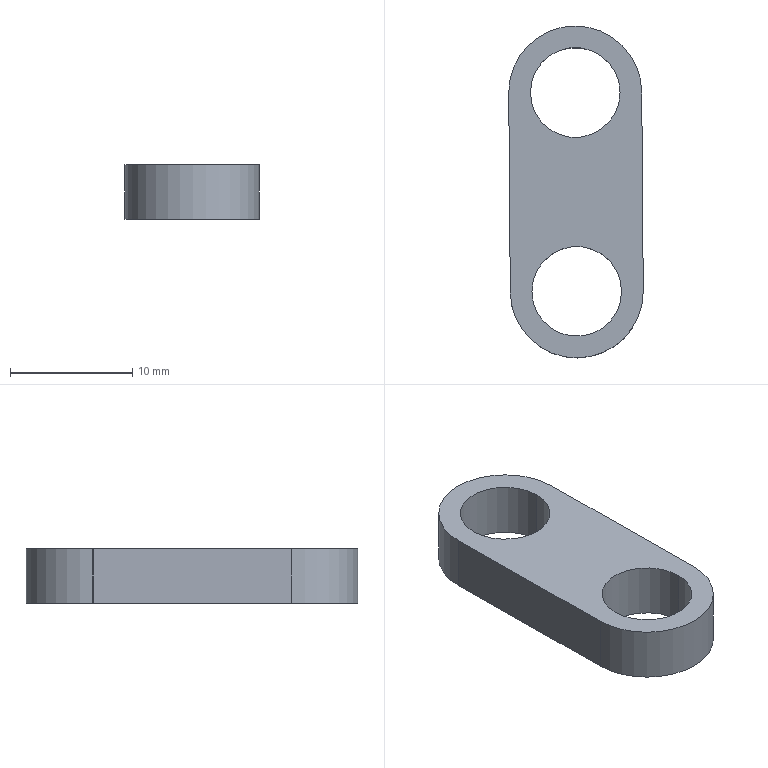Part | SolidWorks | features Extrusion 1 | 1 solid | 11 faces | box 11.013 x 27.178 x 4.5 mm | volume 835.586 mm3 | cylinder 7 | plane 4 | commonest cylinder face diameters 7.349 x4 10.89 x3
STEP:
#1=CARTESIAN_POINT('',(22.577,-16.261,4.5));
#2=VERTEX_POINT('',#1);
#3=CARTESIAN_POINT('',(29.926,-16.261,4.5));
#4=VERTEX_POINT('',#3);
#5=CARTESIAN_POINT('',(26.251,-16.261,4.5));
#6=DIRECTION('',(0.,0.,1.));
#7=DIRECTION('',(1.,0.,0.));
#8=AXIS2_PLACEMENT_3D('',#5,#6,#7);
#9=CIRCLE('',#8,3.675);
#10=EDGE_CURVE('',#2,#4,#9,.T.);
#11=ORIENTED_EDGE('',*,*,#10,.T.);
#12=CARTESIAN_POINT('',(29.926,-16.261,0.));
#13=VERTEX_POINT('',#12);
#14=CARTESIAN_POINT('',(29.926,-16.261,33.825));
#15=DIRECTION('',(0.,0.,-1.));
#16=VECTOR('',#15,1000.);
#17=LINE('',#14,#16);
#18=EDGE_CURVE('',#4,#13,#17,.T.);
#19=ORIENTED_EDGE('',*,*,#18,.T.);
#20=CARTESIAN_POINT('',(22.577,-16.261,0.));
#21=VERTEX_POINT('',#20);
#22=CARTESIAN_POINT('',(26.251,-16.261,0.));
#23=DIRECTION('',(0.,0.,1.));
#24=DIRECTION('',(1.,0.,0.));
#25=AXIS2_PLACEMENT_3D('',#22,#23,#24);
#26=CIRCLE('',#25,3.675);
#27=EDGE_CURVE('',#21,#13,#26,.T.);
#28=ORIENTED_EDGE('',*,*,#27,.F.);
#29=CARTESIAN_POINT('',(22.577,-16.261,33.825));
#30=DIRECTION('',(0.,0.,-1.));
#31=VECTOR('',#30,1000.);
#32=LINE('',#29,#31);
#33=EDGE_CURVE('',#2,#21,#32,.T.);
#34=ORIENTED_EDGE('',*,*,#33,.F.);
#35=EDGE_LOOP('',(#11,#19,#28,#34));
#36=FACE_OUTER_BOUND('',#35,.T.);
#37=CARTESIAN_POINT('',(26.251,-16.261,33.825));
#38=DIRECTION('',(0.,0.,-1.));
#39=DIRECTION('',(-1.,0.,0.));
#40=AXIS2_PLACEMENT_3D('',#37,#38,#39);
#41=CYLINDRICAL_SURFACE('',#40,3.675);
#42=ADVANCED_FACE('',(#36),#41,.F.);
#43=CARTESIAN_POINT('',(20.683,0.027,4.5));
#44=VERTEX_POINT('',#43);
#45=CARTESIAN_POINT('',(20.683,-0.01419,4.5));
#46=VERTEX_POINT('',#45);
#47=CARTESIAN_POINT('',(26.128,0.027,4.5));
#48=DIRECTION('',(0.,0.,1.));
#49=DIRECTION('',(1.,0.,0.));
#50=AXIS2_PLACEMENT_3D('',#47,#48,#49);
#51=CIRCLE('',#50,5.445);
#52=EDGE_CURVE('',#44,#46,#51,.T.);
#53=ORIENTED_EDGE('',*,*,#52,.F.);
#54=CARTESIAN_POINT('',(20.683,0.027,0.));
#55=VERTEX_POINT('',#54);
#56=CARTESIAN_POINT('',(20.683,0.027,33.825));
#57=DIRECTION('',(0.,0.,-1.));
#58=VECTOR('',#57,1000.);
#59=LINE('',#56,#58);
#60=EDGE_CURVE('',#44,#55,#59,.T.);
#61=ORIENTED_EDGE('',*,*,#60,.T.);
#62=CARTESIAN_POINT('',(20.683,-0.01419,0.));
#63=VERTEX_POINT('',#62);
#64=CARTESIAN_POINT('',(26.128,0.027,0.));
#65=DIRECTION('',(0.,0.,1.));
#66=DIRECTION('',(1.,0.,0.));
#67=AXIS2_PLACEMENT_3D('',#64,#65,#66);
#68=CIRCLE('',#67,5.445);
#69=EDGE_CURVE('',#55,#63,#68,.T.);
#70=ORIENTED_EDGE('',*,*,#69,.T.);
#71=CARTESIAN_POINT('',(20.683,-0.01419,33.825));
#72=DIRECTION('',(0.,0.,-1.));
#73=VECTOR('',#72,1000.);
#74=LINE('',#71,#73);
#75=EDGE_CURVE('',#46,#63,#74,.T.);
#76=ORIENTED_EDGE('',*,*,#75,.F.);
#77=EDGE_LOOP('',(#53,#61,#70,#76));
#78=FACE_OUTER_BOUND('',#77,.T.);
#79=CARTESIAN_POINT('',(26.128,0.027,33.825));
#80=DIRECTION('',(0.,0.,-1.));
#81=DIRECTION('',(-1.,0.,0.));
#82=AXIS2_PLACEMENT_3D('',#79,#80,#81);
#83=CYLINDRICAL_SURFACE('',#82,5.445);
#84=ADVANCED_FACE('',(#78),#83,.T.);
#85=CARTESIAN_POINT('',(22.454,0.027,4.5));
#86=VERTEX_POINT('',#85);
#87=CARTESIAN_POINT('',(29.803,0.027,4.5));
#88=VERTEX_POINT('',#87);
#89=CARTESIAN_POINT('',(26.128,0.027,4.5));
#90=DIRECTION('',(0.,0.,1.));
#91=DIRECTION('',(1.,0.,0.));
#92=AXIS2_PLACEMENT_3D('',#89,#90,#91);
#93=CIRCLE('',#92,3.675);
#94=EDGE_CURVE('',#86,#88,#93,.T.);
#95=ORIENTED_EDGE('',*,*,#94,.T.);
#96=CARTESIAN_POINT('',(29.803,0.027,0.));
#97=VERTEX_POINT('',#96);
#98=CARTESIAN_POINT('',(29.803,0.027,33.825));
#99=DIRECTION('',(0.,0.,-1.));
#100=VECTOR('',#99,1000.);
#101=LINE('',#98,#100);
#102=EDGE_CURVE('',#88,#97,#101,.T.);
#103=ORIENTED_EDGE('',*,*,#102,.T.);
#104=CARTESIAN_POINT('',(22.454,0.027,0.));
#105=VERTEX_POINT('',#104);
#106=CARTESIAN_POINT('',(26.128,0.027,0.));
#107=DIRECTION('',(0.,0.,1.));
#108=DIRECTION('',(1.,0.,0.));
#109=AXIS2_PLACEMENT_3D('',#106,#107,#108);
#110=CIRCLE('',#109,3.675);
#111=EDGE_CURVE('',#105,#97,#110,.T.);
#112=ORIENTED_EDGE('',*,*,#111,.F.);
#113=CARTESIAN_POINT('',(22.454,0.027,33.825));
#114=DIRECTION('',(0.,0.,-1.));
#115=VECTOR('',#114,1000.);
#116=LINE('',#113,#115);
#117=EDGE_CURVE('',#86,#105,#116,.T.);
#118=ORIENTED_EDGE('',*,*,#117,.F.);
#119=EDGE_LOOP('',(#95,#103,#112,#118));
#120=FACE_OUTER_BOUND('',#119,.T.);
#121=CARTESIAN_POINT('',(26.128,0.027,33.825));
#122=DIRECTION('',(0.,0.,-1.));
#123=DIRECTION('',(-1.,0.,0.));
#124=AXIS2_PLACEMENT_3D('',#121,#122,#123);
#125=CYLINDRICAL_SURFACE('',#124,3.675);
#126=ADVANCED_FACE('',(#120),#125,.F.);
#127=ORIENTED_EDGE('',*,*,#102,.F.);
#128=CARTESIAN_POINT('',(26.128,0.027,4.5));
#129=DIRECTION('',(0.,0.,1.));
#130=DIRECTION('',(1.,0.,0.));
#131=AXIS2_PLACEMENT_3D('',#128,#129,#130);
#132=CIRCLE('',#131,3.675);
#133=EDGE_CURVE('',#88,#86,#132,.T.);
#134=ORIENTED_EDGE('',*,*,#133,.T.);
#135=ORIENTED_EDGE('',*,*,#117,.T.);
#136=CARTESIAN_POINT('',(26.128,0.027,0.));
#137=DIRECTION('',(0.,0.,1.));
#138=DIRECTION('',(1.,0.,0.));
#139=AXIS2_PLACEMENT_3D('',#136,#137,#138);
#140=CIRCLE('',#139,3.675);
#141=EDGE_CURVE('',#97,#105,#140,.T.);
#142=ORIENTED_EDGE('',*,*,#141,.F.);
#143=EDGE_LOOP('',(#127,#134,#135,#142));
#144=FACE_OUTER_BOUND('',#143,.T.);
#145=CARTESIAN_POINT('',(26.128,0.027,33.825));
#146=DIRECTION('',(0.,0.,-1.));
#147=DIRECTION('',(-1.,0.,0.));
#148=AXIS2_PLACEMENT_3D('',#145,#146,#147);
#149=CYLINDRICAL_SURFACE('',#148,3.675);
#150=ADVANCED_FACE('',(#144),#149,.F.);
#151=CARTESIAN_POINT('',(31.696,-16.22,4.5));
#152=VERTEX_POINT('',#151);
#153=CARTESIAN_POINT('',(31.573,0.06818,4.5));
#154=VERTEX_POINT('',#153);
#155=CARTESIAN_POINT('',(31.696,-16.22,4.5));
#156=DIRECTION('',(-0.007564,1.,0.));
#157=VECTOR('',#156,1000.);
#158=LINE('',#155,#157);
#159=EDGE_CURVE('',#152,#154,#158,.T.);
#160=ORIENTED_EDGE('',*,*,#159,.F.);
#161=CARTESIAN_POINT('',(31.696,-16.22,0.));
#162=VERTEX_POINT('',#161);
#163=CARTESIAN_POINT('',(31.696,-16.22,33.825));
#164=DIRECTION('',(0.,0.,-1.));
#165=VECTOR('',#164,1000.);
#166=LINE('',#163,#165);
#167=EDGE_CURVE('',#152,#162,#166,.T.);
#168=ORIENTED_EDGE('',*,*,#167,.T.);
#169=CARTESIAN_POINT('',(31.573,0.06818,0.));
#170=VERTEX_POINT('',#169);
#171=CARTESIAN_POINT('',(31.696,-16.22,0.));
#172=DIRECTION('',(-0.007564,1.,0.));
#173=VECTOR('',#172,1000.);
#174=LINE('',#171,#173);
#175=EDGE_CURVE('',#162,#170,#174,.T.);
#176=ORIENTED_EDGE('',*,*,#175,.T.);
#177=CARTESIAN_POINT('',(31.573,0.06818,33.825));
#178=DIRECTION('',(0.,0.,-1.));
#179=VECTOR('',#178,1000.);
#180=LINE('',#177,#179);
#181=EDGE_CURVE('',#154,#170,#180,.T.);
#182=ORIENTED_EDGE('',*,*,#181,.F.);
#183=EDGE_LOOP('',(#160,#168,#176,#182));
#184=FACE_OUTER_BOUND('',#183,.T.);
#185=CARTESIAN_POINT('',(31.696,-16.22,33.825));
#186=DIRECTION('',(-1.,-0.007564,0.));
#187=DIRECTION('',(0.007564,-1.,0.));
#188=AXIS2_PLACEMENT_3D('',#185,#186,#187);
#189=PLANE('',#188);
#190=ADVANCED_FACE('',(#184),#189,.F.);
#191=CARTESIAN_POINT('',(20.807,-16.302,4.5));
#192=VERTEX_POINT('',#191);
#193=CARTESIAN_POINT('',(26.251,-16.261,4.5));
#194=DIRECTION('',(0.,0.,1.));
#195=DIRECTION('',(1.,0.,0.));
#196=AXIS2_PLACEMENT_3D('',#193,#194,#195);
#197=CIRCLE('',#196,5.445);
#198=EDGE_CURVE('',#192,#152,#197,.T.);
#199=ORIENTED_EDGE('',*,*,#198,.F.);
#200=CARTESIAN_POINT('',(20.807,-16.302,0.));
#201=VERTEX_POINT('',#200);
#202=CARTESIAN_POINT('',(20.807,-16.302,33.825));
#203=DIRECTION('',(0.,0.,-1.));
#204=VECTOR('',#203,1000.);
#205=LINE('',#202,#204);
#206=EDGE_CURVE('',#192,#201,#205,.T.);
#207=ORIENTED_EDGE('',*,*,#206,.T.);
#208=CARTESIAN_POINT('',(26.251,-16.261,0.));
#209=DIRECTION('',(0.,0.,1.));
#210=DIRECTION('',(1.,0.,0.));
#211=AXIS2_PLACEMENT_3D('',#208,#209,#210);
#212=CIRCLE('',#211,5.445);
#213=EDGE_CURVE('',#201,#162,#212,.T.);
#214=ORIENTED_EDGE('',*,*,#213,.T.);
#215=ORIENTED_EDGE('',*,*,#167,.F.);
#216=EDGE_LOOP('',(#199,#207,#214,#215));
#217=FACE_OUTER_BOUND('',#216,.T.);
#218=CARTESIAN_POINT('',(26.251,-16.261,33.825));
#219=DIRECTION('',(0.,0.,-1.));
#220=DIRECTION('',(-1.,0.,0.));
#221=AXIS2_PLACEMENT_3D('',#218,#219,#220);
#222=CYLINDRICAL_SURFACE('',#221,5.445);
#223=ADVANCED_FACE('',(#217),#222,.T.);
#224=CARTESIAN_POINT('',(20.683,-0.01419,4.5));
#225=DIRECTION('',(0.007564,-1.,0.));
#226=VECTOR('',#225,1000.);
#227=LINE('',#224,#226);
#228=EDGE_CURVE('',#46,#192,#227,.T.);
#229=ORIENTED_EDGE('',*,*,#228,.F.);
#230=ORIENTED_EDGE('',*,*,#75,.T.);
#231=CARTESIAN_POINT('',(20.683,-0.01419,0.));
#232=DIRECTION('',(0.007564,-1.,0.));
#233=VECTOR('',#232,1000.);
#234=LINE('',#231,#233);
#235=EDGE_CURVE('',#63,#201,#234,.T.);
#236=ORIENTED_EDGE('',*,*,#235,.T.);
#237=ORIENTED_EDGE('',*,*,#206,.F.);
#238=EDGE_LOOP('',(#229,#230,#236,#237));
#239=FACE_OUTER_BOUND('',#238,.T.);
#240=CARTESIAN_POINT('',(20.683,-0.01419,33.825));
#241=DIRECTION('',(1.,0.007564,0.));
#242=DIRECTION('',(-0.007564,1.,0.));
#243=AXIS2_PLACEMENT_3D('',#240,#241,#242);
#244=PLANE('',#243);
#245=ADVANCED_FACE('',(#239),#244,.F.);
#246=ORIENTED_EDGE('',*,*,#60,.F.);
#247=CARTESIAN_POINT('',(26.128,0.027,4.5));
#248=DIRECTION('',(0.,0.,1.));
#249=DIRECTION('',(1.,0.,0.));
#250=AXIS2_PLACEMENT_3D('',#247,#248,#249);
#251=CIRCLE('',#250,5.445);
#252=EDGE_CURVE('',#154,#44,#251,.T.);
#253=ORIENTED_EDGE('',*,*,#252,.F.);
#254=ORIENTED_EDGE('',*,*,#181,.T.);
#255=CARTESIAN_POINT('',(26.128,0.027,0.));
#256=DIRECTION('',(0.,0.,1.));
#257=DIRECTION('',(1.,0.,0.));
#258=AXIS2_PLACEMENT_3D('',#255,#256,#257);
#259=CIRCLE('',#258,5.445);
#260=EDGE_CURVE('',#170,#55,#259,.T.);
#261=ORIENTED_EDGE('',*,*,#260,.T.);
#262=EDGE_LOOP('',(#246,#253,#254,#261));
#263=FACE_OUTER_BOUND('',#262,.T.);
#264=CARTESIAN_POINT('',(26.128,0.027,33.825));
#265=DIRECTION('',(0.,0.,-1.));
#266=DIRECTION('',(-1.,0.,0.));
#267=AXIS2_PLACEMENT_3D('',#264,#265,#266);
#268=CYLINDRICAL_SURFACE('',#267,5.445);
#269=ADVANCED_FACE('',(#263),#268,.T.);
#270=ORIENTED_EDGE('',*,*,#260,.F.);
#271=ORIENTED_EDGE('',*,*,#175,.F.);
#272=ORIENTED_EDGE('',*,*,#213,.F.);
#273=ORIENTED_EDGE('',*,*,#235,.F.);
#274=ORIENTED_EDGE('',*,*,#69,.F.);
#275=EDGE_LOOP('',(#270,#271,#272,#273,#274));
#276=FACE_OUTER_BOUND('',#275,.T.);
#277=ORIENTED_EDGE('',*,*,#111,.T.);
#278=ORIENTED_EDGE('',*,*,#141,.T.);
#279=EDGE_LOOP('',(#277,#278));
#280=FACE_BOUND('',#279,.T.);
#281=ORIENTED_EDGE('',*,*,#27,.T.);
#282=CARTESIAN_POINT('',(26.251,-16.261,0.));
#283=DIRECTION('',(0.,0.,1.));
#284=DIRECTION('',(1.,0.,0.));
#285=AXIS2_PLACEMENT_3D('',#282,#283,#284);
#286=CIRCLE('',#285,3.675);
#287=EDGE_CURVE('',#13,#21,#286,.T.);
#288=ORIENTED_EDGE('',*,*,#287,.T.);
#289=EDGE_LOOP('',(#281,#288));
#290=FACE_BOUND('',#289,.T.);
#291=CARTESIAN_POINT('',(26.128,0.027,0.));
#292=DIRECTION('',(0.,0.,1.));
#293=DIRECTION('',(1.,0.,0.));
#294=AXIS2_PLACEMENT_3D('',#291,#292,#293);
#295=PLANE('',#294);
#296=ADVANCED_FACE('',(#276,#280,#290),#295,.F.);
#297=ORIENTED_EDGE('',*,*,#18,.F.);
#298=CARTESIAN_POINT('',(26.251,-16.261,4.5));
#299=DIRECTION('',(0.,0.,1.));
#300=DIRECTION('',(1.,0.,0.));
#301=AXIS2_PLACEMENT_3D('',#298,#299,#300);
#302=CIRCLE('',#301,3.675);
#303=EDGE_CURVE('',#4,#2,#302,.T.);
#304=ORIENTED_EDGE('',*,*,#303,.T.);
#305=ORIENTED_EDGE('',*,*,#33,.T.);
#306=ORIENTED_EDGE('',*,*,#287,.F.);
#307=EDGE_LOOP('',(#297,#304,#305,#306));
#308=FACE_OUTER_BOUND('',#307,.T.);
#309=CARTESIAN_POINT('',(26.251,-16.261,33.825));
#310=DIRECTION('',(0.,0.,-1.));
#311=DIRECTION('',(-1.,0.,0.));
#312=AXIS2_PLACEMENT_3D('',#309,#310,#311);
#313=CYLINDRICAL_SURFACE('',#312,3.675);
#314=ADVANCED_FACE('',(#308),#313,.F.);
#315=ORIENTED_EDGE('',*,*,#10,.F.);
#316=ORIENTED_EDGE('',*,*,#303,.F.);
#317=EDGE_LOOP('',(#315,#316));
#318=FACE_BOUND('',#317,.T.);
#319=ORIENTED_EDGE('',*,*,#94,.F.);
#320=ORIENTED_EDGE('',*,*,#133,.F.);
#321=EDGE_LOOP('',(#319,#320));
#322=FACE_BOUND('',#321,.T.);
#323=ORIENTED_EDGE('',*,*,#159,.T.);
#324=ORIENTED_EDGE('',*,*,#252,.T.);
#325=ORIENTED_EDGE('',*,*,#52,.T.);
#326=ORIENTED_EDGE('',*,*,#228,.T.);
#327=ORIENTED_EDGE('',*,*,#198,.T.);
#328=EDGE_LOOP('',(#323,#324,#325,#326,#327));
#329=FACE_OUTER_BOUND('',#328,.T.);
#330=CARTESIAN_POINT('',(53.194,0.027,4.5));
#331=DIRECTION('',(0.,0.,1.));
#332=DIRECTION('',(1.,0.,0.));
#333=AXIS2_PLACEMENT_3D('',#330,#331,#332);
#334=PLANE('',#333);
#335=ADVANCED_FACE('',(#318,#322,#329),#334,.T.);
#336=CLOSED_SHELL('',(#42,#84,#126,#150,#190,#223,#245,#269,#296,#314,#335));
#337=MANIFOLD_SOLID_BREP('',#336);
#338=CARTESIAN_POINT('',(0.,0.,0.));
#339=DIRECTION('',(0.,0.,1.));
#340=DIRECTION('',(1.,0.,0.));
#341=AXIS2_PLACEMENT_3D('',#338,#339,#340);
#342=(LENGTH_UNIT()NAMED_UNIT(*)SI_UNIT(.MILLI.,.METRE.));
#343=UNCERTAINTY_MEASURE_WITH_UNIT(LENGTH_MEASURE(0.00001),#342,'','');
#344=(NAMED_UNIT(*)PLANE_ANGLE_UNIT()SI_UNIT($,.RADIAN.));
#345=(NAMED_UNIT(*)SI_UNIT($,.STERADIAN.)SOLID_ANGLE_UNIT());
#346=(GEOMETRIC_REPRESENTATION_CONTEXT(3)GLOBAL_UNCERTAINTY_ASSIGNED_CONTEXT((#343))GLOBAL_UNIT_ASSIGNED_CONTEXT((#342,#344,#345))REPRESENTATION_CONTEXT('',''));
#347=ADVANCED_BREP_SHAPE_REPRESENTATION('',(#337,#341),#346);